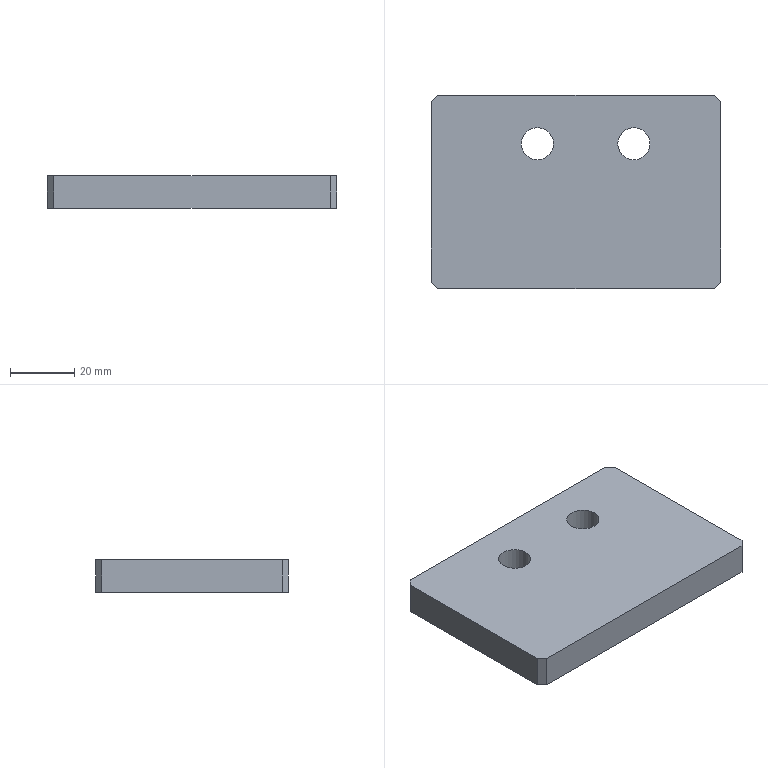NC program | NX | posted with a generic post | part box 90 x 60 x 10 mm
Lines 1 to 539 of 1827:
N10 G17 G21 G94 G90
(PLANAR_MILL , TOOL : D80面刀)
N12 T01 M6
N14 G53
N16 G17 G0 G90 X88. Y0. S2000 M3
N18 G43 Z20. H1
N20 Z2.05
N22 G94 G1 Z0.05 F800.
N24 X43.
N26 X-43.
N28 X-88.
N30 Z2.05
N32 G0 Z20.
N34 M5
(ADAPTIVE_MILLING , TOOL : D12开粗)
N36 T02 M6
N38 G53
N40 G17 G0 G90 X-60.067 Y-28.629 S3000 M3
N42 G43 Z20. H2
N44 Z-8.
N46 G94 G1 X-59.917 Y-28.631 Z-8.937 F1500.
N48 X-59.767 Y-28.632 Z-9.308
N50 X-59.617 Y-28.634 Z-9.58
N52 X-59.467 Y-28.636 Z-9.8
N54 X-59.317 Y-28.638 Z-9.984
N56 X-59.167 Y-28.64 Z-10.142
N58 X-59.017 Y-28.641 Z-10.28
N60 X-58.867 Y-28.643 Z-10.4
N62 X-58.717 Y-28.645 Z-10.505
N64 X-58.567 Y-28.647 Z-10.598
N66 X-58.417 Y-28.649 Z-10.679
N68 X-58.267 Y-28.651 Z-10.75
N70 X-58.117 Y-28.652 Z-10.81
N72 X-57.967 Y-28.654 Z-10.862
N74 X-57.817 Y-28.656 Z-10.905
N76 X-57.667 Y-28.658 Z-10.939
N78 X-57.517 Y-28.66 Z-10.966
N80 X-57.367 Y-28.662 Z-10.985
N82 X-57.217 Y-28.663 Z-10.996
N84 X-57.067 Y-28.665 Z-11.
N86 X-55.212 Y-28.688
N88 G3 X-54.046 Y-27.856 R1.212
N90 X-53.636 Y-25.016 R11.721
N92 X-53.501 Y-15.414 R203.48
N94 G1 X-53.499 Y32.644
N96 G2 X-51.178 Y37.519 R6.599
N98 X-46.513 Y39.805 R10.493
N100 X-40.931 Y40.416 R29.026
N102 X-29.556 Y40.499 R429.914
N104 G1 X45.814 Y40.497
N106 G2 X50.631 Y38.05 R6.673
N108 X52.843 Y33.347 R10.709
N110 X53.427 Y27.573 R30.997
N112 X53.499 Y15.324 R579.839
N114 G1 X53.496 Y-32.812
N116 G2 X51.097 Y-37.588 R6.66
N118 X46.347 Y-39.841 R10.673
N120 X40.76 Y-40.421 R30.356
N122 X29.573 Y-40.499 R462.276
N124 G1 X-45.762 Y-40.498
N126 G2 X-50.596 Y-38.088 R6.65
N128 X-52.844 Y-33.336 R10.679
N130 X-53.279 Y-29.368 R17.794
N132 G1 X-53.275 Y24.119
N134 G3 X-53.025 Y29.579 R53.052
N136 G2 X-52.457 Y33.307 R9.621
N138 X-47.94 Y38.077 R9.196
N140 X-42.427 Y39.619 R16.56
N142 X-35.502 Y39.97 R65.227
N144 G1 X-26.315 Y39.998
N146 X43.455 Y39.997
N148 G2 X50.337 Y36.175 R8.478
N150 X52.422 Y30.728 R13.749
N152 X52.945 Y23.88 R45.056
N154 X52.998 Y12.88 R718.904
N156 G1 X52.997 Y-30.454
N158 G2 X49.294 Y-37.253 R8.462
N160 X43.923 Y-39.386 R13.489
N162 X37.515 Y-39.933 R40.942
N164 X26.016 Y-39.999 R648.707
N166 G1 X-43.453 Y-39.997
N168 G2 X-50.256 Y-36.29 R8.463
N170 X-52.334 Y-30.845 R12.635
N172 X-52.738 Y-24.8 R44.631
N174 X-52.778 Y-13.926 R737.561
N176 G1 X-52.775 Y24.112
N178 G3 X-52.523 Y29.293 R283.84
N180 G2 X-47.62 Y37.004 R9.764
N182 X-41.906 Y38.94 R16.045
N184 X-34.742 Y39.447 R52.534
N186 X-23.68 Y39.498 R719.978
N188 G1 X41.455 Y39.496
N190 G2 X50.028 Y34.554 R9.72
N192 X51.948 Y28.838 R16.086
N194 X52.448 Y21.486 R54.058
N196 X52.498 Y9.361 R774.066
N198 G1 Y-28.203
N200 G2 X50.195 Y-34.839 R9.758
N202 X44.76 Y-38.266 R11.828
N204 X38.486 Y-39.304 R26.069
N206 X27.739 Y-39.496 R191.872
N208 G1 X23.614 Y-39.498
N210 X-41.453 Y-39.496
N212 G2 X-50.217 Y-34.164 R9.671
N214 X-51.863 Y-28.556 R16.509
N216 X-52.249 Y-21.071 R65.024
N218 G1 X-52.278 Y-10.696
N220 Y24.005
N222 G2 X-52.02 Y28.311 R87.923
N224 X-46.324 Y36.585 R10.702
N226 X-40.268 Y38.465 R18.02
N228 X-32.413 Y38.955 R62.376
N230 X-21.789 Y38.998 R725.415
N232 G1 X39.455 Y38.997
N234 G2 X44.518 Y38.069 R12.22
N236 X49.861 Y32.747 R10.943
N238 X51.555 Y26.562 R19.397
N240 X51.963 Y18.514 R74.548
N242 G1 X51.997 Y7.264
N244 Y-26.266
N246 G2 X51.282 Y-30.996 R12.961
N248 X45.902 Y-36.783 R10.813
N250 X39.861 Y-38.517 R18.843
N252 X32.065 Y-38.96 R67.46
N254 X21.753 Y-38.998 R728.596
N256 G1 X-39.485 Y-38.996
N258 G2 X-44.545 Y-38.055 R12.11
N260 X-49.834 Y-32.65 R10.747
N262 X-51.093 Y-28.892 R22.174
N264 X-51.707 Y-21.488 R47.606
N266 X-51.778 Y-8.363 R763.002
N268 G1 Y24.049
N270 G2 X-51.346 Y28.329 R25.536
N272 X-45.426 Y36.003 R11.387
N274 X-39.185 Y37.929 R18.974
N276 X-31.333 Y38.444 R62.131
N278 X-18.958 Y38.497 R769.388
N280 G1 X37.78 Y38.496
N282 G2 X42.593 Y37.869 R15.308
N284 X48.566 Y33.133 R11.267
N286 X50.114 Y31.415 R12.738
N288 G1 X50.682 Y30.352
N290 X51.032 Y29.198
N292 G2 X51.176 Y26.686 R21.34
N294 X51.491 Y12.051 R273.552
N296 G1 X51.497 Y5.551
N298 X51.495 Y-24.749
N300 G2 X51.053 Y-28.98 R16.78
N302 G1 X51.031 Y-29.201
N304 G2 X49.022 Y-33.075 R9.27
N306 X43.096 Y-36.997 R13.098
N308 X36.539 Y-38.22 R26.734
N310 X26.92 Y-38.487 R136.965
N312 G1 X18.92 Y-38.497
N314 X-37.703 Y-38.496
N316 G2 X-42.4 Y-37.927 R15.66
N318 X-48.352 Y-33.345 R11.026
N320 X-50.114 Y-31.415 R15.861
N322 G1 X-50.7 Y-30.292
N324 X-51.032 Y-29.198
N326 X-51.15 Y-28.
N328 G3 X-51.248 Y-18.274 R517.249
N330 G1 X-51.277 Y-7.149
N332 X-51.266 Y24.2
N334 X-51.15 Y25.57
N336 Y28.001
N338 X-51.031 Y29.201
N340 X-50.681 Y30.355
N342 X-50.113 Y31.418
N344 X-49.348 Y32.349
N346 X-47.348 Y34.349
N348 X-46.415 Y35.114
N350 G2 X-44.054 Y36.135 R9.339
N352 X-34.912 Y37.763 R35.662
N354 X-24.041 Y37.99 R193.493
N356 G1 X-17.041 Y37.997
N358 X39.072 Y37.993
N360 G2 X44.64 Y35.908 R13.072
N362 G1 X45.355 Y35.681
N364 X46.418 Y35.113
N366 G2 X48.587 Y33.111 R18.704
N368 G3 X50.599 Y33.667 R1.2
N370 X50.515 Y34.495 Z-10.964 R1.289
N372 G1 X49.972 Y35.93 Z-10.9
N374 X49.271 Y37.779 F15000.
N376 G3 X48.587 Y38.471 R1.202
N378 G1 X43.739 Y40.371
N380 G3 X39.449 Y41.392 R15.82
N382 X35.005 Y41.601 R48.24
N384 G1 X-23.671 Y41.636
N386 G3 X-35.734 Y41.321 R235.876
N388 X-40.081 Y40.791 R38.613
N390 G1 X-42.672 Y40.324
N392 G3 X-43.156 Y40.12 R1.228
N394 G1 X-44.784 Y38.958
N396 X-46.449 Y37.766 Z-10.986 F1500.
N398 X-46.572 Y37.652 Z-10.993
N400 X-46.679 Y37.525 Z-11.
N402 G3 X-45.352 Y35.682 R1.2
N404 G1 X-44.198 Y36.032
N406 G3 X-39.929 Y36.669 R75.076
N408 G2 X-29.653 Y37.426 R77.68
N410 X-16.028 Y37.496 R785.741
N412 G1 X39.084 Y37.493
N414 G2 X42.668 Y36.22 R19.435
N416 G1 X43.001 Y36.15
N418 X44.201 Y36.031
N420 X44.739 Y35.868
N422 G3 X46.104 Y37.655 R1.2
N424 X45.634 Y38.091 Z-10.973 R1.338
N426 G1 X44.17 Y39.022 Z-10.9
N428 X43.035 Y39.743 F15000.
N430 G3 X42.394 Y39.93 R1.21
N432 G1 X-41.293 Y40.149
N434 G3 X-41.97 Y39.942 R1.209
N436 G1 X-43.17 Y39.128
N438 X-44.486 Y38.231 Z-10.967 F1500.
N440 G3 X-44.917 Y37.587 Z-11. R1.202
N442 X-43.639 Y36.087 R1.2
N444 G2 X-41.684 Y36.155 R14.847
N446 G3 X-35.854 Y36.622 R244.853
N448 G2 X-23.675 Y36.98 R180.749
N450 G1 X-14.05 Y36.996
N452 X39.125 Y36.992
N454 G2 X40.189 Y36.636 R5.651
N456 G3 X41.629 Y36.154 R8.551
N458 G1 X43.001 Y36.15
N460 G3 X44.193 Y37.482 R1.2
N462 X43.601 Y38.395 Z-10.953 R1.255
N464 G1 X42.578 Y39.121 Z-10.9
N466 X41.349 Y39.991 F15000.
N468 G3 X40.656 Y40.212 R1.208
N470 G1 X-39.529
N472 G3 X-40.223 Y39.991 R1.208
N474 G1 X-41.426 Y39.139
N476 X-42.031 Y38.712 Z-10.931 F1500.
N478 X-42.631 Y38.277 Z-10.962
N480 G3 X-43.063 Y37.512 Z-11. R1.2
N482 X-41.874 Y36.15 R1.2
N484 X-31.693 Y36.338 R173.678
N486 G2 X-12.82 Y36.496 R652.241
N488 G1 X38.043 Y36.492
N490 X39.595 Y36.15
N492 X41.72
N494 G3 X42.913 Y37.477 R1.2
N496 X42.323 Y38.393 Z-10.953 R1.255
N498 G1 X41.302 Y39.121 Z-10.9
N500 X40.083 Y39.989 F15000.
N502 G3 X39.375 Y40.212 R1.207
N504 G1 X-33.87 Y39.466
N506 X-34.025 Y39.453
N508 X-34.177 Y39.423
N510 X-35.234 Y39.132
N512 X-37.531 Y38.5 Z-11. F1500.
N514 G3 X-37.187 Y36.15 R1.2
N516 G1 X43.001
N518 X44.201 Y36.031
N520 X45.355 Y35.681
N522 X46.418 Y35.113
N524 X47.349 Y34.348
N526 X49.349 Y32.348
N528 X50.114 Y31.415
N530 X50.682 Y30.352
N532 X51.032 Y29.198
N534 G2 X51.15 Y27.562 R10.821
N536 G1 Y-28.001
N538 X51.031 Y-29.201
N540 X50.681 Y-30.355
N542 X50.113 Y-31.418
N544 X49.348 Y-32.349
N546 X47.348 Y-34.349
N548 X46.415 Y-35.114
N550 G2 X44.112 Y-36.112 R9.157
N552 X35.157 Y-37.744 R35.41
N554 X23.912 Y-37.99 R185.952
N556 G1 X17.037 Y-37.997
N558 X-39.065 Y-37.994
N560 G2 X-44.518 Y-35.952 R12.634
N562 G1 X-45.355 Y-35.681
N564 X-46.418 Y-35.113
N566 G2 X-48.366 Y-33.332 R16.117
N568 G3 X-50.395 Y-33.966 R1.2
N570 X-50.285 Y-34.734 Z-10.967 R1.303
N572 G1 X-49.689 Y-36.213 Z-10.9
N574 X-48.942 Y-38.067 F15000.
N576 G3 X-48.366 Y-38.692 R1.204
N578 G1 X-47.12 Y-39.318
N580 X-45.868 Y-39.931
N582 G3 X-41.901 Y-41.18 R16.765
N584 X-36.915 Y-41.666 R25.458
N586 G1 X28.328 Y-41.572
N588 G3 X35.725 Y-41.232 R83.436
N590 G1 X38.59 Y-40.963
N592 G3 X41.044 Y-40.611 R42.485
N594 G1 X42.672 Y-40.324
N596 G3 X43.162 Y-40.119 R1.227
N598 G1 X44.788 Y-38.957
N600 X46.45 Y-37.765 Z-10.986 F1500.
N602 X46.573 Y-37.651 Z-10.993
N604 X46.681 Y-37.522 Z-11.
N606 G3 X45.352 Y-35.682 R1.2
N608 G1 X44.198 Y-36.032
N610 G3 X40.237 Y-36.618 R60.702
N612 G2 X29.839 Y-37.421 R75.899
N614 X15.464 Y-37.497 R807.051
N616 G1 X-39.073 Y-37.493
N618 G2 X-42.655 Y-36.214 R20.072
N620 G3 X-44.201 Y-36.031 R11.433
N622 G1 X-44.68 Y-35.886
N624 G3 X-46.058 Y-37.65 R1.2
N626 X-45.576 Y-38.108 Z-10.972 R1.327
N628 G1 X-44.133 Y-39.025 Z-10.9
N630 X-42.975 Y-39.761 F15000.
N632 G3 X-42.335 Y-39.948 R1.21
N634 G1 X41.231 Y-40.155
N636 G3 X41.908 Y-39.948 R1.209
N638 G1 X43.113 Y-39.131
N640 X44.425 Y-38.237 Z-10.967 F1500.
N642 G3 X44.856 Y-37.587 Z-11. R1.202
N644 X43.576 Y-36.093 R1.2
N646 G2 X41.634 Y-36.155 R15.398
N648 G3 X35.856 Y-36.619 R257.993
N650 G2 X23.614 Y-36.98 R181.195
N652 G1 X13.989 Y-36.996
N654 X-39.111 Y-36.993
N656 G2 X-40.444 Y-36.531 R7.427
N658 G3 X-41.663 Y-36.15 R5.314
N660 G1 X-42.976
N662 G3 X-44.169 Y-37.482 R1.2
N664 X-43.577 Y-38.395 Z-10.953 R1.255
N666 G1 X-42.553 Y-39.121 Z-10.9
N668 X-41.325 Y-39.991 F15000.
N670 G3 X-40.631 Y-40.212 R1.208
N672 G1 X39.467
N674 G3 X40.16 Y-39.991 R1.208
N676 G1 X41.363 Y-39.139
N678 X41.969 Y-38.712 Z-10.931 F1500.
N680 X42.569 Y-38.277 Z-10.962
N682 G3 X43.001 Y-37.512 Z-11. R1.2
N684 X41.812 Y-36.15 R1.2
N686 X31.82 Y-36.333 R168.72
N688 G2 X12.821 Y-36.496 R641.866
N690 G1 X-38.028 Y-36.492
N692 X-39.573 Y-36.15
N694 X-41.698
N696 G3 X-42.891 Y-37.477 R1.2
N698 X-42.301 Y-38.393 Z-10.953 R1.255
N700 G1 X-41.28 Y-39.121 Z-10.9
N702 X-40.061 Y-39.989 F15000.
N704 G3 X-39.353 Y-40.212 R1.207
N706 G1 X33.87 Y-39.466
N708 X34.025 Y-39.453
N710 X34.177 Y-39.423
N712 X35.234 Y-39.132
N714 X37.531 Y-38.5 Z-11. F1500.
N716 G3 X37.187 Y-36.15 R1.2
N718 G1 X-43.001
N720 X-44.201 Y-36.031
N722 X-45.355 Y-35.681
N724 X-46.418 Y-35.113
N726 X-47.349 Y-34.348
N728 X-49.349 Y-32.348
N730 X-50.114 Y-31.415
N732 X-50.682 Y-30.352
N734 X-51.032 Y-29.198
N736 X-51.15 Y-28.
N738 Y25.625
N740 G3 X-52.301 Y26.835 R1.212
N742 G1 X-54.128 Y26.927
N744 X-54.278 Y26.935 Z-10.996
N746 X-54.427 Y26.942 Z-10.985
N748 X-54.577 Y26.95 Z-10.966
N750 X-54.727 Y26.957 Z-10.939
N752 X-54.877 Y26.965 Z-10.905
N754 X-55.027 Y26.972 Z-10.862
N756 X-55.177 Y26.98 Z-10.81
N758 X-55.326 Y26.987 Z-10.75
N760 X-55.476 Y26.995 Z-10.679
N762 X-55.626 Y27.002 Z-10.598
N764 X-55.776 Y27.01 Z-10.505
N766 X-55.926 Y27.017 Z-10.4
N768 X-56.075 Y27.025 Z-10.28
N770 X-56.225 Y27.032 Z-10.142
N772 X-56.375 Y27.04 Z-9.984
N774 X-56.525 Y27.047 Z-9.8
N776 X-56.675 Y27.055 Z-9.58
N778 X-56.824 Y27.062 Z-9.308
N780 X-56.974 Y27.07 Z-8.937
N782 X-57.124 Y27.077 Z-8.
N784 G0 Z20.
N786 M5
(PLANAR_MILL_1 , TOOL : D10精光)
N788 T03 M6
N790 G53
N792 G17 G0 G90 X-40.071 Y-40. S3000 M3
N794 G43 Z20. H3
N796 Z-8.
N798 G94 G1 Z-11. F800.
N800 X-46.536 Y-33.535
N802 X-48.536 Y-31.536
N804 G2 X-50. Y-28. R5.
N806 G1 Y28.
N808 G2 X-48.536 Y31.536 R5.
N810 G1 X-46.536 Y33.536
N812 G2 X-43. Y35. R5.
N814 G1 X43.
N816 G2 X46.536 Y33.536 R5.
N818 G1 X48.536 Y31.536
N820 G2 X50. Y28. R5.
N822 G1 Y-28.
N824 G2 X48.536 Y-31.536 R5.
N826 G1 X46.536 Y-33.536
N828 G2 X43. Y-35. R5.
N830 G1 X-42.999
N832 X-52.141
N834 Z-8.
N836 G0 Z20.
N838 X-40.071 Y-40.
N840 Z-8.
N842 G1 Z-11.
N844 X-46.536 Y-33.535
N846 X-48.536 Y-31.536
N848 G2 X-50. Y-28. R5.
N850 G1 Y28.
N852 G2 X-48.536 Y31.536 R5.
N854 G1 X-46.536 Y33.536
N856 G2 X-43. Y35. R5.
N858 G1 X43.
N860 G2 X46.536 Y33.536 R5.
N862 G1 X48.536 Y31.536
N864 G2 X50. Y28. R5.
N866 G1 Y-28.
N868 G2 X48.536 Y-31.536 R5.
N870 G1 X46.536 Y-33.536
N872 G2 X43. Y-35. R5.
N874 G1 X-42.999
N876 X-52.141
N878 Z-8.
N880 G0 Z20.
N882 M5
(SPOT_DRILLING , TOOL : D6倒角刀)
N884 T05 M6
N886 G53
N888 G17 G0 G90 X-12. Y15. S2000 M3
N890 G43 Z20. H5
N892 G94 G81 G98 Z-1. F150. R3.
N894 X18.
N896 G80
N898 M5
(SPOT_DRILLING_COPY , TOOL : D8.6钻头)
N900 T06 M6
N902 G53
N904 G17 G0 G90 X-12. Y15. S1600 M3
N906 G43 Z20. H6
N908 G94 G83 G98 Z-17. F100. Q1.889 R3.
N910 X18.
N912 G80
N914 M5
(PLANAR_MILL_1_COPY , TOOL : D6倒角刀)
N916 T05 M6
N918 G53
N920 G17 G0 G90 X-40.414 Y-34. S3000 M3
N922 G43 Z20. H5
N924 Z2.
N926 G94 G1 Z-1. F800.
N928 X-43.707 Y-30.707
N930 X-45.707 Y-28.707
N932 G2 X-46. Y-28. R1.
N934 G1 Y28.
N936 G2 X-45.707 Y28.707 R1.
N938 G1 X-43.707 Y30.707
N940 G2 X-43. Y31. R1.
N942 G1 X43.
N944 G2 X43.707 Y30.707 R1.
N946 G1 X45.707 Y28.707
N948 G2 X46. Y28. R1.
N950 G1 Y-28.
N952 G2 X45.707 Y-28.707 R1.
N954 G1 X43.707 Y-30.707
N956 G2 X43. Y-31. R1.
N958 G1 X-43.
N960 X-47.657
N962 Z2.
N964 G0 Z20.
(PLANAR_MILL_1_COPY_COPY , TOOL : D6倒角刀)
N966 X-13.101 Y16.295
N968 Z0.5
N970 G1 Z-1.5
N972 X-13.7 Y17.
N974 G3 X-15.7 Y15. R2.
N976 X-12. Y11.3 R3.7
N978 X-15.7 Y15. R-3.7
N980 X-13.7 Y13. R2.
N982 G1 X-13.101 Y13.705
N984 Z0.5
N986 G0 Z20.
N988 X16.899 Y16.295
N990 Z0.5
N992 G1 Z-1.5
N994 X16.3 Y17.
N996 G3 X14.3 Y15. R2.
N998 X18. Y11.3 R3.7
N1000 X14.3 Y15. R-3.7
N1002 X16.3 Y13. R2.
N1004 G1 X16.899 Y13.705
N1006 Z0.5
N1008 G0 Z20.
N1010 M5
(PLANAR_MILL_COPY , TOOL : D80面刀)
N1012 T01 M6
N1014 G53
N1016 G17 G0 G90 X88. Y0. S2000 M3
N1018 G43 Z20. H1
N1020 Z2.
N1022 G94 G1 Z0. F800.
N1024 X43.
N1026 X-43.
N1028 X-88.
N1030 Z2.
N1032 G0 Z20.
N1034 M5